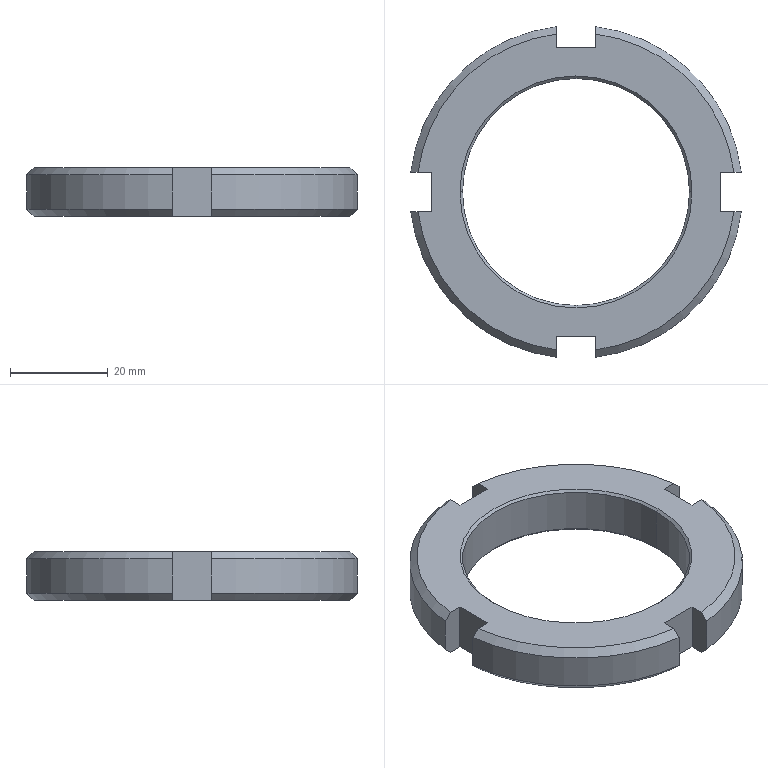Part | SolidWorks | features BaseBody 1 | 1 solid | 32 faces | box 67.528 x 67.528 x 10 mm | volume 17576 mm3 | plane 14 | cone 12 | cylinder 6 | commonest cylinder face diameters 68 x4 46.376 x2
STEP:
#1=CARTESIAN_POINT('',(-23.188,0.,9.5));
#2=VERTEX_POINT('',#1);
#3=CARTESIAN_POINT('',(23.188,0.,9.5));
#4=VERTEX_POINT('',#3);
#5=CARTESIAN_POINT('',(0.,0.,9.5));
#6=DIRECTION('',(0.,0.,1.));
#7=DIRECTION('',(1.,0.,0.));
#8=AXIS2_PLACEMENT_3D('',#5,#6,#7);
#9=CIRCLE('',#8,23.188);
#10=EDGE_CURVE('',#2,#4,#9,.T.);
#11=ORIENTED_EDGE('',*,*,#10,.F.);
#12=CARTESIAN_POINT('',(-23.688,0.,10.));
#13=VERTEX_POINT('',#12);
#14=CARTESIAN_POINT('',(-23.188,0.,9.5));
#15=DIRECTION('',(-0.7071,0.,0.7071));
#16=VECTOR('',#15,1000.);
#17=LINE('',#14,#16);
#18=EDGE_CURVE('',#2,#13,#17,.T.);
#19=ORIENTED_EDGE('',*,*,#18,.T.);
#20=CARTESIAN_POINT('',(23.688,0.,10.));
#21=VERTEX_POINT('',#20);
#22=CARTESIAN_POINT('',(0.,0.,10.));
#23=DIRECTION('',(0.,0.,-1.));
#24=DIRECTION('',(1.,0.,0.));
#25=AXIS2_PLACEMENT_3D('',#22,#23,#24);
#26=CIRCLE('',#25,23.688);
#27=EDGE_CURVE('',#21,#13,#26,.T.);
#28=ORIENTED_EDGE('',*,*,#27,.F.);
#29=CARTESIAN_POINT('',(23.188,0.,9.5));
#30=DIRECTION('',(0.7071,0.,0.7071));
#31=VECTOR('',#30,1000.);
#32=LINE('',#29,#31);
#33=EDGE_CURVE('',#4,#21,#32,.T.);
#34=ORIENTED_EDGE('',*,*,#33,.F.);
#35=EDGE_LOOP('',(#11,#19,#28,#34));
#36=FACE_OUTER_BOUND('',#35,.T.);
#37=CARTESIAN_POINT('',(0.,0.,9.5));
#38=DIRECTION('',(0.,0.,1.));
#39=DIRECTION('',(1.,0.,0.));
#40=AXIS2_PLACEMENT_3D('',#37,#38,#39);
#41=CONICAL_SURFACE('',#40,23.188,0.7854);
#42=ADVANCED_FACE('',(#36),#41,.F.);
#43=CARTESIAN_POINT('',(23.188,0.,0.5));
#44=VERTEX_POINT('',#43);
#45=CARTESIAN_POINT('',(-23.188,0.,0.5));
#46=VERTEX_POINT('',#45);
#47=CARTESIAN_POINT('',(0.,0.,0.5));
#48=DIRECTION('',(0.,0.,-1.));
#49=DIRECTION('',(1.,0.,0.));
#50=AXIS2_PLACEMENT_3D('',#47,#48,#49);
#51=CIRCLE('',#50,23.188);
#52=EDGE_CURVE('',#44,#46,#51,.T.);
#53=ORIENTED_EDGE('',*,*,#52,.F.);
#54=CARTESIAN_POINT('',(23.688,0.,0.));
#55=VERTEX_POINT('',#54);
#56=CARTESIAN_POINT('',(23.688,0.,0.));
#57=DIRECTION('',(0.7071,0.,-0.7071));
#58=VECTOR('',#57,1000.);
#59=LINE('',#56,#58);
#60=EDGE_CURVE('',#44,#55,#59,.T.);
#61=ORIENTED_EDGE('',*,*,#60,.T.);
#62=CARTESIAN_POINT('',(-23.688,0.,0.));
#63=VERTEX_POINT('',#62);
#64=CARTESIAN_POINT('',(0.,0.,0.));
#65=DIRECTION('',(0.,0.,1.));
#66=DIRECTION('',(1.,0.,0.));
#67=AXIS2_PLACEMENT_3D('',#64,#65,#66);
#68=CIRCLE('',#67,23.688);
#69=EDGE_CURVE('',#63,#55,#68,.T.);
#70=ORIENTED_EDGE('',*,*,#69,.F.);
#71=CARTESIAN_POINT('',(-23.688,0.,0.));
#72=DIRECTION('',(-0.7071,0.,-0.7071));
#73=VECTOR('',#72,1000.);
#74=LINE('',#71,#73);
#75=EDGE_CURVE('',#46,#63,#74,.T.);
#76=ORIENTED_EDGE('',*,*,#75,.F.);
#77=EDGE_LOOP('',(#53,#61,#70,#76));
#78=FACE_OUTER_BOUND('',#77,.T.);
#79=CARTESIAN_POINT('',(0.,0.,0.));
#80=DIRECTION('',(0.,0.,-1.));
#81=DIRECTION('',(-1.,0.,0.));
#82=AXIS2_PLACEMENT_3D('',#79,#80,#81);
#83=CONICAL_SURFACE('',#82,23.688,0.7854);
#84=ADVANCED_FACE('',(#78),#83,.F.);
#85=ORIENTED_EDGE('',*,*,#10,.T.);
#86=CARTESIAN_POINT('',(23.188,0.,10.));
#87=DIRECTION('',(0.,0.,-1.));
#88=VECTOR('',#87,1000.);
#89=LINE('',#86,#88);
#90=EDGE_CURVE('',#4,#44,#89,.T.);
#91=ORIENTED_EDGE('',*,*,#90,.T.);
#92=ORIENTED_EDGE('',*,*,#52,.T.);
#93=CARTESIAN_POINT('',(-23.188,0.,10.));
#94=DIRECTION('',(0.,0.,-1.));
#95=VECTOR('',#94,1000.);
#96=LINE('',#93,#95);
#97=EDGE_CURVE('',#2,#46,#96,.T.);
#98=ORIENTED_EDGE('',*,*,#97,.F.);
#99=EDGE_LOOP('',(#85,#91,#92,#98));
#100=FACE_OUTER_BOUND('',#99,.T.);
#101=CARTESIAN_POINT('',(0.,0.,10.));
#102=DIRECTION('',(0.,0.,-1.));
#103=DIRECTION('',(-1.,0.,0.));
#104=AXIS2_PLACEMENT_3D('',#101,#102,#103);
#105=CYLINDRICAL_SURFACE('',#104,23.188);
#106=ADVANCED_FACE('',(#100),#105,.F.);
#107=CARTESIAN_POINT('',(4.,33.764,8.5));
#108=VERTEX_POINT('',#107);
#109=CARTESIAN_POINT('',(33.764,4.,8.5));
#110=VERTEX_POINT('',#109);
#111=CARTESIAN_POINT('',(0.,0.,8.5));
#112=DIRECTION('',(0.,0.,-1.));
#113=DIRECTION('',(1.,0.,0.));
#114=AXIS2_PLACEMENT_3D('',#111,#112,#113);
#115=CIRCLE('',#114,34.);
#116=EDGE_CURVE('',#108,#110,#115,.T.);
#117=ORIENTED_EDGE('',*,*,#116,.T.);
#118=CARTESIAN_POINT('',(33.764,4.,1.5));
#119=VERTEX_POINT('',#118);
#120=CARTESIAN_POINT('',(33.764,4.,0.));
#121=DIRECTION('',(0.,0.,1.));
#122=VECTOR('',#121,1000.);
#123=LINE('',#120,#122);
#124=EDGE_CURVE('',#119,#110,#123,.T.);
#125=ORIENTED_EDGE('',*,*,#124,.F.);
#126=CARTESIAN_POINT('',(4.,33.764,1.5));
#127=VERTEX_POINT('',#126);
#128=CARTESIAN_POINT('',(0.,0.,1.5));
#129=DIRECTION('',(0.,0.,1.));
#130=DIRECTION('',(1.,0.,0.));
#131=AXIS2_PLACEMENT_3D('',#128,#129,#130);
#132=CIRCLE('',#131,34.);
#133=EDGE_CURVE('',#119,#127,#132,.T.);
#134=ORIENTED_EDGE('',*,*,#133,.T.);
#135=CARTESIAN_POINT('',(4.,33.764,0.));
#136=DIRECTION('',(0.,0.,1.));
#137=VECTOR('',#136,1000.);
#138=LINE('',#135,#137);
#139=EDGE_CURVE('',#127,#108,#138,.T.);
#140=ORIENTED_EDGE('',*,*,#139,.T.);
#141=EDGE_LOOP('',(#117,#125,#134,#140));
#142=FACE_OUTER_BOUND('',#141,.T.);
#143=CARTESIAN_POINT('',(0.,0.,10.));
#144=DIRECTION('',(0.,0.,-1.));
#145=DIRECTION('',(-1.,0.,0.));
#146=AXIS2_PLACEMENT_3D('',#143,#144,#145);
#147=CYLINDRICAL_SURFACE('',#146,34.);
#148=ADVANCED_FACE('',(#142),#147,.T.);
#149=CARTESIAN_POINT('',(32.253,4.,10.));
#150=VERTEX_POINT('',#149);
#151=CARTESIAN_POINT('',(33.764,4.,8.5));
#152=CARTESIAN_POINT('',(33.371,4.,8.89));
#153=CARTESIAN_POINT('',(32.979,4.,9.28));
#154=CARTESIAN_POINT('',(32.586,4.,9.669));
#155=CARTESIAN_POINT('',(32.475,4.,9.779));
#156=CARTESIAN_POINT('',(32.364,4.,9.89));
#157=CARTESIAN_POINT('',(32.253,4.,10.));
#158=B_SPLINE_CURVE_WITH_KNOTS('',3,(#151,#152,#153,#154,#155,#156,#157),.UNSPECIFIED.,.F.,.F.,(4,3,4),(0.007216,0.008875,0.009345),.UNSPECIFIED.);
#159=EDGE_CURVE('',#110,#150,#158,.T.);
#160=ORIENTED_EDGE('',*,*,#159,.F.);
#161=ORIENTED_EDGE('',*,*,#116,.F.);
#162=CARTESIAN_POINT('',(4.,32.253,10.));
#163=VERTEX_POINT('',#162);
#164=CARTESIAN_POINT('',(4.,32.253,10.));
#165=CARTESIAN_POINT('',(4.,32.364,9.89));
#166=CARTESIAN_POINT('',(4.,32.475,9.779));
#167=CARTESIAN_POINT('',(4.,32.586,9.669));
#168=CARTESIAN_POINT('',(4.,32.979,9.28));
#169=CARTESIAN_POINT('',(4.,33.371,8.89));
#170=CARTESIAN_POINT('',(4.,33.764,8.5));
#171=B_SPLINE_CURVE_WITH_KNOTS('',3,(#164,#165,#166,#167,#168,#169,#170),.UNSPECIFIED.,.F.,.F.,(4,3,4),(0.008406,0.008875,0.01053),.UNSPECIFIED.);
#172=EDGE_CURVE('',#163,#108,#171,.T.);
#173=ORIENTED_EDGE('',*,*,#172,.F.);
#174=CARTESIAN_POINT('',(0.,0.,10.));
#175=DIRECTION('',(0.,0.,1.));
#176=DIRECTION('',(1.,0.,0.));
#177=AXIS2_PLACEMENT_3D('',#174,#175,#176);
#178=CIRCLE('',#177,32.5);
#179=EDGE_CURVE('',#150,#163,#178,.T.);
#180=ORIENTED_EDGE('',*,*,#179,.F.);
#181=EDGE_LOOP('',(#160,#161,#173,#180));
#182=FACE_OUTER_BOUND('',#181,.T.);
#183=CARTESIAN_POINT('',(0.,0.,10.));
#184=DIRECTION('',(0.,0.,-1.));
#185=DIRECTION('',(-1.,0.,0.));
#186=AXIS2_PLACEMENT_3D('',#183,#184,#185);
#187=CONICAL_SURFACE('',#186,32.5,0.7854);
#188=ADVANCED_FACE('',(#182),#187,.T.);
#189=CARTESIAN_POINT('',(32.253,4.,0.));
#190=VERTEX_POINT('',#189);
#191=CARTESIAN_POINT('',(32.253,4.,0.));
#192=CARTESIAN_POINT('',(32.364,4.,0.1102));
#193=CARTESIAN_POINT('',(32.475,4.,0.2205));
#194=CARTESIAN_POINT('',(32.586,4.,0.3308));
#195=CARTESIAN_POINT('',(32.979,4.,0.7205));
#196=CARTESIAN_POINT('',(33.371,4.,1.11));
#197=CARTESIAN_POINT('',(33.764,4.,1.5));
#198=B_SPLINE_CURVE_WITH_KNOTS('',3,(#191,#192,#193,#194,#195,#196,#197),.UNSPECIFIED.,.F.,.F.,(4,3,4),(0.008406,0.008875,0.01053),.UNSPECIFIED.);
#199=EDGE_CURVE('',#190,#119,#198,.T.);
#200=ORIENTED_EDGE('',*,*,#199,.F.);
#201=CARTESIAN_POINT('',(4.,32.253,0.));
#202=VERTEX_POINT('',#201);
#203=CARTESIAN_POINT('',(0.,0.,0.));
#204=DIRECTION('',(0.,0.,-1.));
#205=DIRECTION('',(1.,0.,0.));
#206=AXIS2_PLACEMENT_3D('',#203,#204,#205);
#207=CIRCLE('',#206,32.5);
#208=EDGE_CURVE('',#202,#190,#207,.T.);
#209=ORIENTED_EDGE('',*,*,#208,.F.);
#210=CARTESIAN_POINT('',(4.,33.764,1.5));
#211=CARTESIAN_POINT('',(4.,33.371,1.11));
#212=CARTESIAN_POINT('',(4.,32.979,0.7205));
#213=CARTESIAN_POINT('',(4.,32.586,0.3308));
#214=CARTESIAN_POINT('',(4.,32.475,0.2205));
#215=CARTESIAN_POINT('',(4.,32.364,0.1102));
#216=CARTESIAN_POINT('',(4.,32.253,0.));
#217=B_SPLINE_CURVE_WITH_KNOTS('',3,(#210,#211,#212,#213,#214,#215,#216),.UNSPECIFIED.,.F.,.F.,(4,3,4),(0.007216,0.008875,0.009345),.UNSPECIFIED.);
#218=EDGE_CURVE('',#127,#202,#217,.T.);
#219=ORIENTED_EDGE('',*,*,#218,.F.);
#220=ORIENTED_EDGE('',*,*,#133,.F.);
#221=EDGE_LOOP('',(#200,#209,#219,#220));
#222=FACE_OUTER_BOUND('',#221,.T.);
#223=CARTESIAN_POINT('',(0.,0.,1.5));
#224=DIRECTION('',(0.,0.,1.));
#225=DIRECTION('',(1.,0.,0.));
#226=AXIS2_PLACEMENT_3D('',#223,#224,#225);
#227=CONICAL_SURFACE('',#226,34.,0.7854);
#228=ADVANCED_FACE('',(#222),#227,.T.);
#229=CARTESIAN_POINT('',(-33.764,4.,8.5));
#230=VERTEX_POINT('',#229);
#231=CARTESIAN_POINT('',(-4.,33.764,8.5));
#232=VERTEX_POINT('',#231);
#233=CARTESIAN_POINT('',(0.,0.,8.5));
#234=DIRECTION('',(0.,0.,-1.));
#235=DIRECTION('',(1.,0.,0.));
#236=AXIS2_PLACEMENT_3D('',#233,#234,#235);
#237=CIRCLE('',#236,34.);
#238=EDGE_CURVE('',#230,#232,#237,.T.);
#239=ORIENTED_EDGE('',*,*,#238,.T.);
#240=CARTESIAN_POINT('',(-4.,33.764,1.5));
#241=VERTEX_POINT('',#240);
#242=CARTESIAN_POINT('',(-4.,33.764,0.));
#243=DIRECTION('',(0.,0.,1.));
#244=VECTOR('',#243,1000.);
#245=LINE('',#242,#244);
#246=EDGE_CURVE('',#241,#232,#245,.T.);
#247=ORIENTED_EDGE('',*,*,#246,.F.);
#248=CARTESIAN_POINT('',(-33.764,4.,1.5));
#249=VERTEX_POINT('',#248);
#250=CARTESIAN_POINT('',(0.,0.,1.5));
#251=DIRECTION('',(0.,0.,1.));
#252=DIRECTION('',(1.,0.,0.));
#253=AXIS2_PLACEMENT_3D('',#250,#251,#252);
#254=CIRCLE('',#253,34.);
#255=EDGE_CURVE('',#241,#249,#254,.T.);
#256=ORIENTED_EDGE('',*,*,#255,.T.);
#257=CARTESIAN_POINT('',(-33.764,4.,0.));
#258=DIRECTION('',(0.,0.,1.));
#259=VECTOR('',#258,1000.);
#260=LINE('',#257,#259);
#261=EDGE_CURVE('',#249,#230,#260,.T.);
#262=ORIENTED_EDGE('',*,*,#261,.T.);
#263=EDGE_LOOP('',(#239,#247,#256,#262));
#264=FACE_OUTER_BOUND('',#263,.T.);
#265=CARTESIAN_POINT('',(0.,0.,10.));
#266=DIRECTION('',(0.,0.,-1.));
#267=DIRECTION('',(-1.,0.,0.));
#268=AXIS2_PLACEMENT_3D('',#265,#266,#267);
#269=CYLINDRICAL_SURFACE('',#268,34.);
#270=ADVANCED_FACE('',(#264),#269,.T.);
#271=CARTESIAN_POINT('',(-4.,32.253,10.));
#272=VERTEX_POINT('',#271);
#273=CARTESIAN_POINT('',(-4.,33.764,8.5));
#274=CARTESIAN_POINT('',(-4.,33.371,8.89));
#275=CARTESIAN_POINT('',(-4.,32.979,9.28));
#276=CARTESIAN_POINT('',(-4.,32.586,9.669));
#277=CARTESIAN_POINT('',(-4.,32.475,9.779));
#278=CARTESIAN_POINT('',(-4.,32.364,9.89));
#279=CARTESIAN_POINT('',(-4.,32.253,10.));
#280=B_SPLINE_CURVE_WITH_KNOTS('',3,(#273,#274,#275,#276,#277,#278,#279),.UNSPECIFIED.,.F.,.F.,(4,3,4),(0.007216,0.008875,0.009345),.UNSPECIFIED.);
#281=EDGE_CURVE('',#232,#272,#280,.T.);
#282=ORIENTED_EDGE('',*,*,#281,.F.);
#283=ORIENTED_EDGE('',*,*,#238,.F.);
#284=CARTESIAN_POINT('',(-32.253,4.,10.));
#285=VERTEX_POINT('',#284);
#286=CARTESIAN_POINT('',(-32.253,4.,10.));
#287=CARTESIAN_POINT('',(-32.542,4.,9.713));
#288=CARTESIAN_POINT('',(-32.832,4.,9.425));
#289=CARTESIAN_POINT('',(-33.121,4.,9.138));
#290=CARTESIAN_POINT('',(-33.336,4.,8.925));
#291=CARTESIAN_POINT('',(-33.55,4.,8.713));
#292=CARTESIAN_POINT('',(-33.764,4.,8.5));
#293=B_SPLINE_CURVE_WITH_KNOTS('',3,(#286,#287,#288,#289,#290,#291,#292),.UNSPECIFIED.,.F.,.F.,(4,3,4),(0.007652,0.008875,0.009781),.UNSPECIFIED.);
#294=EDGE_CURVE('',#285,#230,#293,.T.);
#295=ORIENTED_EDGE('',*,*,#294,.F.);
#296=CARTESIAN_POINT('',(0.,0.,10.));
#297=DIRECTION('',(0.,0.,1.));
#298=DIRECTION('',(1.,0.,0.));
#299=AXIS2_PLACEMENT_3D('',#296,#297,#298);
#300=CIRCLE('',#299,32.5);
#301=EDGE_CURVE('',#272,#285,#300,.T.);
#302=ORIENTED_EDGE('',*,*,#301,.F.);
#303=EDGE_LOOP('',(#282,#283,#295,#302));
#304=FACE_OUTER_BOUND('',#303,.T.);
#305=CARTESIAN_POINT('',(0.,0.,10.));
#306=DIRECTION('',(0.,0.,-1.));
#307=DIRECTION('',(-1.,0.,0.));
#308=AXIS2_PLACEMENT_3D('',#305,#306,#307);
#309=CONICAL_SURFACE('',#308,32.5,0.7854);
#310=ADVANCED_FACE('',(#304),#309,.T.);
#311=CARTESIAN_POINT('',(-4.,32.253,0.));
#312=VERTEX_POINT('',#311);
#313=CARTESIAN_POINT('',(-4.,32.253,0.));
#314=CARTESIAN_POINT('',(-4.,32.364,0.1102));
#315=CARTESIAN_POINT('',(-4.,32.475,0.2205));
#316=CARTESIAN_POINT('',(-4.,32.586,0.3308));
#317=CARTESIAN_POINT('',(-4.,32.979,0.7205));
#318=CARTESIAN_POINT('',(-4.,33.371,1.11));
#319=CARTESIAN_POINT('',(-4.,33.764,1.5));
#320=B_SPLINE_CURVE_WITH_KNOTS('',3,(#313,#314,#315,#316,#317,#318,#319),.UNSPECIFIED.,.F.,.F.,(4,3,4),(0.008406,0.008875,0.01053),.UNSPECIFIED.);
#321=EDGE_CURVE('',#312,#241,#320,.T.);
#322=ORIENTED_EDGE('',*,*,#321,.F.);
#323=CARTESIAN_POINT('',(-32.253,4.,0.));
#324=VERTEX_POINT('',#323);
#325=CARTESIAN_POINT('',(0.,0.,0.));
#326=DIRECTION('',(0.,0.,-1.));
#327=DIRECTION('',(1.,0.,0.));
#328=AXIS2_PLACEMENT_3D('',#325,#326,#327);
#329=CIRCLE('',#328,32.5);
#330=EDGE_CURVE('',#324,#312,#329,.T.);
#331=ORIENTED_EDGE('',*,*,#330,.F.);
#332=CARTESIAN_POINT('',(-33.764,4.,1.5));
#333=CARTESIAN_POINT('',(-33.55,4.,1.287));
#334=CARTESIAN_POINT('',(-33.336,4.,1.075));
#335=CARTESIAN_POINT('',(-33.121,4.,0.8621));
#336=CARTESIAN_POINT('',(-32.832,4.,0.5747));
#337=CARTESIAN_POINT('',(-32.542,4.,0.2873));
#338=CARTESIAN_POINT('',(-32.253,4.,0.));
#339=B_SPLINE_CURVE_WITH_KNOTS('',3,(#332,#333,#334,#335,#336,#337,#338),.UNSPECIFIED.,.F.,.F.,(4,3,4),(0.00797,0.008875,0.0101),.UNSPECIFIED.);
#340=EDGE_CURVE('',#249,#324,#339,.T.);
#341=ORIENTED_EDGE('',*,*,#340,.F.);
#342=ORIENTED_EDGE('',*,*,#255,.F.);
#343=EDGE_LOOP('',(#322,#331,#341,#342));
#344=FACE_OUTER_BOUND('',#343,.T.);
#345=CARTESIAN_POINT('',(0.,0.,1.5));
#346=DIRECTION('',(0.,0.,1.));
#347=DIRECTION('',(1.,0.,0.));
#348=AXIS2_PLACEMENT_3D('',#345,#346,#347);
#349=CONICAL_SURFACE('',#348,34.,0.7854);
#350=ADVANCED_FACE('',(#344),#349,.T.);
#351=CARTESIAN_POINT('',(-4.,-33.764,8.5));
#352=VERTEX_POINT('',#351);
#353=CARTESIAN_POINT('',(-33.764,-4.,8.5));
#354=VERTEX_POINT('',#353);
#355=CARTESIAN_POINT('',(0.,0.,8.5));
#356=DIRECTION('',(0.,0.,-1.));
#357=DIRECTION('',(1.,0.,0.));
#358=AXIS2_PLACEMENT_3D('',#355,#356,#357);
#359=CIRCLE('',#358,34.);
#360=EDGE_CURVE('',#352,#354,#359,.T.);
#361=ORIENTED_EDGE('',*,*,#360,.T.);
#362=CARTESIAN_POINT('',(-33.764,-4.,1.5));
#363=VERTEX_POINT('',#362);
#364=CARTESIAN_POINT('',(-33.764,-4.,0.));
#365=DIRECTION('',(0.,0.,1.));
#366=VECTOR('',#365,1000.);
#367=LINE('',#364,#366);
#368=EDGE_CURVE('',#363,#354,#367,.T.);
#369=ORIENTED_EDGE('',*,*,#368,.F.);
#370=CARTESIAN_POINT('',(-4.,-33.764,1.5));
#371=VERTEX_POINT('',#370);
#372=CARTESIAN_POINT('',(0.,0.,1.5));
#373=DIRECTION('',(0.,0.,1.));
#374=DIRECTION('',(1.,0.,0.));
#375=AXIS2_PLACEMENT_3D('',#372,#373,#374);
#376=CIRCLE('',#375,34.);
#377=EDGE_CURVE('',#363,#371,#376,.T.);
#378=ORIENTED_EDGE('',*,*,#377,.T.);
#379=CARTESIAN_POINT('',(-4.,-33.764,0.));
#380=DIRECTION('',(0.,0.,1.));
#381=VECTOR('',#380,1000.);
#382=LINE('',#379,#381);
#383=EDGE_CURVE('',#371,#352,#382,.T.);
#384=ORIENTED_EDGE('',*,*,#383,.T.);
#385=EDGE_LOOP('',(#361,#369,#378,#384));
#386=FACE_OUTER_BOUND('',#385,.T.);
#387=CARTESIAN_POINT('',(0.,0.,10.));
#388=DIRECTION('',(0.,0.,-1.));
#389=DIRECTION('',(-1.,0.,0.));
#390=AXIS2_PLACEMENT_3D('',#387,#388,#389);
#391=CYLINDRICAL_SURFACE('',#390,34.);
#392=ADVANCED_FACE('',(#386),#391,.T.);
#393=CARTESIAN_POINT('',(-32.253,-4.,10.));
#394=VERTEX_POINT('',#393);
#395=CARTESIAN_POINT('',(-33.764,-4.,8.5));
#396=CARTESIAN_POINT('',(-33.55,-4.,8.713));
#397=CARTESIAN_POINT('',(-33.336,-4.,8.925));
#398=CARTESIAN_POINT('',(-33.121,-4.,9.138));
#399=CARTESIAN_POINT('',(-32.832,-4.,9.425));
#400=CARTESIAN_POINT('',(-32.542,-4.,9.713));
#401=CARTESIAN_POINT('',(-32.253,-4.,10.));
#402=B_SPLINE_CURVE_WITH_KNOTS('',3,(#395,#396,#397,#398,#399,#400,#401),.UNSPECIFIED.,.F.,.F.,(4,3,4),(0.00797,0.008875,0.0101),.UNSPECIFIED.);
#403=EDGE_CURVE('',#354,#394,#402,.T.);
#404=ORIENTED_EDGE('',*,*,#403,.F.);
#405=ORIENTED_EDGE('',*,*,#360,.F.);
#406=CARTESIAN_POINT('',(-4.,-32.253,10.));
#407=VERTEX_POINT('',#406);
#408=CARTESIAN_POINT('',(-4.,-32.253,10.));
#409=CARTESIAN_POINT('',(-4.,-32.757,9.5));
#410=CARTESIAN_POINT('',(-4.,-33.26,9.));
#411=CARTESIAN_POINT('',(-4.,-33.764,8.5));
#412=B_SPLINE_CURVE_WITH_KNOTS('',3,(#408,#409,#410,#411),.UNSPECIFIED.,.F.,.F.,(4,4),(0.,0.002129),.UNSPECIFIED.);
#413=EDGE_CURVE('',#407,#352,#412,.T.);
#414=ORIENTED_EDGE('',*,*,#413,.F.);
#415=CARTESIAN_POINT('',(0.,0.,10.));
#416=DIRECTION('',(0.,0.,1.));
#417=DIRECTION('',(1.,0.,0.));
#418=AXIS2_PLACEMENT_3D('',#415,#416,#417);
#419=CIRCLE('',#418,32.5);
#420=EDGE_CURVE('',#394,#407,#419,.T.);
#421=ORIENTED_EDGE('',*,*,#420,.F.);
#422=EDGE_LOOP('',(#404,#405,#414,#421));
#423=FACE_OUTER_BOUND('',#422,.T.);
#424=CARTESIAN_POINT('',(0.,0.,10.));
#425=DIRECTION('',(0.,0.,-1.));
#426=DIRECTION('',(-1.,0.,0.));
#427=AXIS2_PLACEMENT_3D('',#424,#425,#426);
#428=CONICAL_SURFACE('',#427,32.5,0.7854);
#429=ADVANCED_FACE('',(#423),#428,.T.);
#430=CARTESIAN_POINT('',(-32.253,-4.,0.));
#431=VERTEX_POINT('',#430);
#432=CARTESIAN_POINT('',(-32.253,-4.,0.));
#433=CARTESIAN_POINT('',(-32.542,-4.,0.2873));
#434=CARTESIAN_POINT('',(-32.832,-4.,0.5747));
#435=CARTESIAN_POINT('',(-33.121,-4.,0.8621));
#436=CARTESIAN_POINT('',(-33.336,-4.,1.075));
#437=CARTESIAN_POINT('',(-33.55,-4.,1.287));
#438=CARTESIAN_POINT('',(-33.764,-4.,1.5));
#439=B_SPLINE_CURVE_WITH_KNOTS('',3,(#432,#433,#434,#435,#436,#437,#438),.UNSPECIFIED.,.F.,.F.,(4,3,4),(0.007652,0.008875,0.009781),.UNSPECIFIED.);
#440=EDGE_CURVE('',#431,#363,#439,.T.);
#441=ORIENTED_EDGE('',*,*,#440,.F.);
#442=CARTESIAN_POINT('',(-4.,-32.253,0.));
#443=VERTEX_POINT('',#442);
#444=CARTESIAN_POINT('',(0.,0.,0.));
#445=DIRECTION('',(0.,0.,-1.));
#446=DIRECTION('',(1.,0.,0.));
#447=AXIS2_PLACEMENT_3D('',#444,#445,#446);
#448=CIRCLE('',#447,32.5);
#449=EDGE_CURVE('',#443,#431,#448,.T.);
#450=ORIENTED_EDGE('',*,*,#449,.F.);
#451=CARTESIAN_POINT('',(-4.,-33.764,1.5));
#452=CARTESIAN_POINT('',(-4.,-33.26,0.9999));
#453=CARTESIAN_POINT('',(-4.,-32.757,0.4999));
#454=CARTESIAN_POINT('',(-4.,-32.253,0.));
#455=B_SPLINE_CURVE_WITH_KNOTS('',3,(#451,#452,#453,#454),.UNSPECIFIED.,.F.,.F.,(4,4),(0.,0.002129),.UNSPECIFIED.);
#456=EDGE_CURVE('',#371,#443,#455,.T.);
#457=ORIENTED_EDGE('',*,*,#456,.F.);
#458=ORIENTED_EDGE('',*,*,#377,.F.);
#459=EDGE_LOOP('',(#441,#450,#457,#458));
#460=FACE_OUTER_BOUND('',#459,.T.);
#461=CARTESIAN_POINT('',(0.,0.,1.5));
#462=DIRECTION('',(0.,0.,1.));
#463=DIRECTION('',(1.,0.,0.));
#464=AXIS2_PLACEMENT_3D('',#461,#462,#463);
#465=CONICAL_SURFACE('',#464,34.,0.7854);
#466=ADVANCED_FACE('',(#460),#465,.T.);
#467=ORIENTED_EDGE('',*,*,#27,.T.);
#468=CARTESIAN_POINT('',(0.,0.,10.));
#469=DIRECTION('',(0.,0.,-1.));
#470=DIRECTION('',(1.,0.,0.));
#471=AXIS2_PLACEMENT_3D('',#468,#469,#470);
#472=CIRCLE('',#471,23.688);
#473=EDGE_CURVE('',#13,#21,#472,.T.);
#474=ORIENTED_EDGE('',*,*,#473,.T.);
#475=EDGE_LOOP('',(#467,#474));
#476=FACE_BOUND('',#475,.T.);
#477=CARTESIAN_POINT('',(29.514,4.,10.));
#478=VERTEX_POINT('',#477);
#479=CARTESIAN_POINT('',(29.514,4.,10.));
#480=DIRECTION('',(-1.,0.,0.));
#481=VECTOR('',#480,1000.);
#482=LINE('',#479,#481);
#483=EDGE_CURVE('',#150,#478,#482,.T.);
#484=ORIENTED_EDGE('',*,*,#483,.F.);
#485=ORIENTED_EDGE('',*,*,#179,.T.);
#486=CARTESIAN_POINT('',(4.,29.514,10.));
#487=VERTEX_POINT('',#486);
#488=CARTESIAN_POINT('',(4.,29.514,10.));
#489=DIRECTION('',(0.,1.,0.));
#490=VECTOR('',#489,1000.);
#491=LINE('',#488,#490);
#492=EDGE_CURVE('',#487,#163,#491,.T.);
#493=ORIENTED_EDGE('',*,*,#492,.F.);
#494=CARTESIAN_POINT('',(-4.,29.514,10.));
#495=VERTEX_POINT('',#494);
#496=CARTESIAN_POINT('',(4.,29.514,10.));
#497=DIRECTION('',(1.,0.,0.));
#498=VECTOR('',#497,1000.);
#499=LINE('',#496,#498);
#500=EDGE_CURVE('',#495,#487,#499,.T.);
#501=ORIENTED_EDGE('',*,*,#500,.F.);
#502=CARTESIAN_POINT('',(-4.,29.514,10.));
#503=DIRECTION('',(0.,-1.,0.));
#504=VECTOR('',#503,1000.);
#505=LINE('',#502,#504);
#506=EDGE_CURVE('',#272,#495,#505,.T.);
#507=ORIENTED_EDGE('',*,*,#506,.F.);
#508=ORIENTED_EDGE('',*,*,#301,.T.);
#509=CARTESIAN_POINT('',(-29.514,4.,10.));
#510=VERTEX_POINT('',#509);
#511=CARTESIAN_POINT('',(-29.514,4.,10.));
#512=DIRECTION('',(-1.,0.,0.));
#513=VECTOR('',#512,1000.);
#514=LINE('',#511,#513);
#515=EDGE_CURVE('',#510,#285,#514,.T.);
#516=ORIENTED_EDGE('',*,*,#515,.F.);
#517=CARTESIAN_POINT('',(-29.514,-4.,10.));
#518=VERTEX_POINT('',#517);
#519=CARTESIAN_POINT('',(-29.514,4.,10.));
#520=DIRECTION('',(0.,1.,0.));
#521=VECTOR('',#520,1000.);
#522=LINE('',#519,#521);
#523=EDGE_CURVE('',#518,#510,#522,.T.);
#524=ORIENTED_EDGE('',*,*,#523,.F.);
#525=CARTESIAN_POINT('',(-29.514,-4.,10.));
#526=DIRECTION('',(1.,0.,0.));
#527=VECTOR('',#526,1000.);
#528=LINE('',#525,#527);
#529=EDGE_CURVE('',#394,#518,#528,.T.);
#530=ORIENTED_EDGE('',*,*,#529,.F.);
#531=ORIENTED_EDGE('',*,*,#420,.T.);
#532=CARTESIAN_POINT('',(-4.,-29.514,10.));
#533=VERTEX_POINT('',#532);
#534=CARTESIAN_POINT('',(-4.,-29.514,10.));
#535=DIRECTION('',(0.,-1.,0.));
#536=VECTOR('',#535,1000.);
#537=LINE('',#534,#536);
#538=EDGE_CURVE('',#533,#407,#537,.T.);
#539=ORIENTED_EDGE('',*,*,#538,.F.);
#540=CARTESIAN_POINT('',(4.,-29.514,10.));
#541=VERTEX_POINT('',#540);
#542=CARTESIAN_POINT('',(-4.,-29.514,10.));
#543=DIRECTION('',(-1.,0.,0.));
#544=VECTOR('',#543,1000.);
#545=LINE('',#542,#544);
#546=EDGE_CURVE('',#541,#533,#545,.T.);
#547=ORIENTED_EDGE('',*,*,#546,.F.);
#548=CARTESIAN_POINT('',(4.,-32.253,10.));
#549=VERTEX_POINT('',#548);
#550=CARTESIAN_POINT('',(4.,-29.514,10.));
#551=DIRECTION('',(0.,1.,0.));
#552=VECTOR('',#551,1000.);
#553=LINE('',#550,#552);
#554=EDGE_CURVE('',#549,#541,#553,.T.);
#555=ORIENTED_EDGE('',*,*,#554,.F.);
#556=CARTESIAN_POINT('',(32.253,-4.,10.));
#557=VERTEX_POINT('',#556);
#558=CARTESIAN_POINT('',(0.,0.,10.));
#559=DIRECTION('',(0.,0.,1.));
#560=DIRECTION('',(1.,0.,0.));
#561=AXIS2_PLACEMENT_3D('',#558,#559,#560);
#562=CIRCLE('',#561,32.5);
#563=EDGE_CURVE('',#549,#557,#562,.T.);
#564=ORIENTED_EDGE('',*,*,#563,.T.);
#565=CARTESIAN_POINT('',(29.514,-4.,10.));
#566=VERTEX_POINT('',#565);
#567=CARTESIAN_POINT('',(29.514,-4.,10.));
#568=DIRECTION('',(1.,0.,0.));
#569=VECTOR('',#568,1000.);
#570=LINE('',#567,#569);
#571=EDGE_CURVE('',#566,#557,#570,.T.);
#572=ORIENTED_EDGE('',*,*,#571,.F.);
#573=CARTESIAN_POINT('',(29.514,-4.,10.));
#574=DIRECTION('',(0.,-1.,0.));
#575=VECTOR('',#574,1000.);
#576=LINE('',#573,#575);
#577=EDGE_CURVE('',#478,#566,#576,.T.);
#578=ORIENTED_EDGE('',*,*,#577,.F.);
#579=EDGE_LOOP('',(#484,#485,#493,#501,#507,#508,#516,#524,#530,#531,#539,#547,#555,#564,#572,#578));
#580=FACE_OUTER_BOUND('',#579,.T.);
#581=CARTESIAN_POINT('',(0.,0.,10.));
#582=DIRECTION('',(0.,0.,1.));
#583=DIRECTION('',(1.,0.,0.));
#584=AXIS2_PLACEMENT_3D('',#581,#582,#583);
#585=PLANE('',#584);
#586=ADVANCED_FACE('',(#476,#580),#585,.T.);
#587=ORIENTED_EDGE('',*,*,#69,.T.);
#588=CARTESIAN_POINT('',(0.,0.,0.));
#589=DIRECTION('',(0.,0.,1.));
#590=DIRECTION('',(1.,0.,0.));
#591=AXIS2_PLACEMENT_3D('',#588,#589,#590);
#592=CIRCLE('',#591,23.688);
#593=EDGE_CURVE('',#55,#63,#592,.T.);
#594=ORIENTED_EDGE('',*,*,#593,.T.);
#595=EDGE_LOOP('',(#587,#594));
#596=FACE_BOUND('',#595,.T.);
#597=ORIENTED_EDGE('',*,*,#208,.T.);
#598=CARTESIAN_POINT('',(29.514,4.,0.));
#599=VERTEX_POINT('',#598);
#600=CARTESIAN_POINT('',(29.514,4.,0.));
#601=DIRECTION('',(-1.,0.,0.));
#602=VECTOR('',#601,1000.);
#603=LINE('',#600,#602);
#604=EDGE_CURVE('',#190,#599,#603,.T.);
#605=ORIENTED_EDGE('',*,*,#604,.T.);
#606=CARTESIAN_POINT('',(29.514,-4.,0.));
#607=VERTEX_POINT('',#606);
#608=CARTESIAN_POINT('',(29.514,-4.,0.));
#609=DIRECTION('',(0.,-1.,0.));
#610=VECTOR('',#609,1000.);
#611=LINE('',#608,#610);
#612=EDGE_CURVE('',#599,#607,#611,.T.);
#613=ORIENTED_EDGE('',*,*,#612,.T.);
#614=CARTESIAN_POINT('',(32.253,-4.,0.));
#615=VERTEX_POINT('',#614);
#616=CARTESIAN_POINT('',(29.514,-4.,0.));
#617=DIRECTION('',(1.,0.,0.));
#618=VECTOR('',#617,1000.);
#619=LINE('',#616,#618);
#620=EDGE_CURVE('',#607,#615,#619,.T.);
#621=ORIENTED_EDGE('',*,*,#620,.T.);
#622=CARTESIAN_POINT('',(4.,-32.253,0.));
#623=VERTEX_POINT('',#622);
#624=CARTESIAN_POINT('',(0.,0.,0.));
#625=DIRECTION('',(0.,0.,-1.));
#626=DIRECTION('',(1.,0.,0.));
#627=AXIS2_PLACEMENT_3D('',#624,#625,#626);
#628=CIRCLE('',#627,32.5);
#629=EDGE_CURVE('',#615,#623,#628,.T.);
#630=ORIENTED_EDGE('',*,*,#629,.T.);
#631=CARTESIAN_POINT('',(4.,-29.514,0.));
#632=VERTEX_POINT('',#631);
#633=CARTESIAN_POINT('',(4.,-29.514,0.));
#634=DIRECTION('',(0.,1.,0.));
#635=VECTOR('',#634,1000.);
#636=LINE('',#633,#635);
#637=EDGE_CURVE('',#623,#632,#636,.T.);
#638=ORIENTED_EDGE('',*,*,#637,.T.);
#639=CARTESIAN_POINT('',(-4.,-29.514,0.));
#640=VERTEX_POINT('',#639);
#641=CARTESIAN_POINT('',(-4.,-29.514,0.));
#642=DIRECTION('',(-1.,0.,0.));
#643=VECTOR('',#642,1000.);
#644=LINE('',#641,#643);
#645=EDGE_CURVE('',#632,#640,#644,.T.);
#646=ORIENTED_EDGE('',*,*,#645,.T.);
#647=CARTESIAN_POINT('',(-4.,-29.514,0.));
#648=DIRECTION('',(0.,-1.,0.));
#649=VECTOR('',#648,1000.);
#650=LINE('',#647,#649);
#651=EDGE_CURVE('',#640,#443,#650,.T.);
#652=ORIENTED_EDGE('',*,*,#651,.T.);
#653=ORIENTED_EDGE('',*,*,#449,.T.);
#654=CARTESIAN_POINT('',(-29.514,-4.,0.));
#655=VERTEX_POINT('',#654);
#656=CARTESIAN_POINT('',(-29.514,-4.,0.));
#657=DIRECTION('',(1.,0.,0.));
#658=VECTOR('',#657,1000.);
#659=LINE('',#656,#658);
#660=EDGE_CURVE('',#431,#655,#659,.T.);
#661=ORIENTED_EDGE('',*,*,#660,.T.);
#662=CARTESIAN_POINT('',(-29.514,4.,0.));
#663=VERTEX_POINT('',#662);
#664=CARTESIAN_POINT('',(-29.514,4.,0.));
#665=DIRECTION('',(0.,1.,0.));
#666=VECTOR('',#665,1000.);
#667=LINE('',#664,#666);
#668=EDGE_CURVE('',#655,#663,#667,.T.);
#669=ORIENTED_EDGE('',*,*,#668,.T.);
#670=CARTESIAN_POINT('',(-29.514,4.,0.));
#671=DIRECTION('',(-1.,0.,0.));
#672=VECTOR('',#671,1000.);
#673=LINE('',#670,#672);
#674=EDGE_CURVE('',#663,#324,#673,.T.);
#675=ORIENTED_EDGE('',*,*,#674,.T.);
#676=ORIENTED_EDGE('',*,*,#330,.T.);
#677=CARTESIAN_POINT('',(-4.,29.514,0.));
#678=VERTEX_POINT('',#677);
#679=CARTESIAN_POINT('',(-4.,29.514,0.));
#680=DIRECTION('',(0.,-1.,0.));
#681=VECTOR('',#680,1000.);
#682=LINE('',#679,#681);
#683=EDGE_CURVE('',#312,#678,#682,.T.);
#684=ORIENTED_EDGE('',*,*,#683,.T.);
#685=CARTESIAN_POINT('',(4.,29.514,0.));
#686=VERTEX_POINT('',#685);
#687=CARTESIAN_POINT('',(4.,29.514,0.));
#688=DIRECTION('',(1.,0.,0.));
#689=VECTOR('',#688,1000.);
#690=LINE('',#687,#689);
#691=EDGE_CURVE('',#678,#686,#690,.T.);
#692=ORIENTED_EDGE('',*,*,#691,.T.);
#693=CARTESIAN_POINT('',(4.,29.514,0.));
#694=DIRECTION('',(0.,1.,0.));
#695=VECTOR('',#694,1000.);
#696=LINE('',#693,#695);
#697=EDGE_CURVE('',#686,#202,#696,.T.);
#698=ORIENTED_EDGE('',*,*,#697,.T.);
#699=EDGE_LOOP('',(#597,#605,#613,#621,#630,#638,#646,#652,#653,#661,#669,#675,#676,#684,#692,#698));
#700=FACE_OUTER_BOUND('',#699,.T.);
#701=CARTESIAN_POINT('',(0.,0.,0.));
#702=DIRECTION('',(0.,0.,1.));
#703=DIRECTION('',(1.,0.,0.));
#704=AXIS2_PLACEMENT_3D('',#701,#702,#703);
#705=PLANE('',#704);
#706=ADVANCED_FACE('',(#596,#700),#705,.F.);
#707=CARTESIAN_POINT('',(4.,-33.764,1.5));
#708=VERTEX_POINT('',#707);
#709=CARTESIAN_POINT('',(33.764,-4.,1.5));
#710=VERTEX_POINT('',#709);
#711=CARTESIAN_POINT('',(0.,0.,1.5));
#712=DIRECTION('',(0.,0.,1.));
#713=DIRECTION('',(1.,0.,0.));
#714=AXIS2_PLACEMENT_3D('',#711,#712,#713);
#715=CIRCLE('',#714,34.);
#716=EDGE_CURVE('',#708,#710,#715,.T.);
#717=ORIENTED_EDGE('',*,*,#716,.T.);
#718=CARTESIAN_POINT('',(33.764,-4.,8.5));
#719=VERTEX_POINT('',#718);
#720=CARTESIAN_POINT('',(33.764,-4.,0.));
#721=DIRECTION('',(0.,0.,1.));
#722=VECTOR('',#721,1000.);
#723=LINE('',#720,#722);
#724=EDGE_CURVE('',#710,#719,#723,.T.);
#725=ORIENTED_EDGE('',*,*,#724,.T.);
#726=CARTESIAN_POINT('',(4.,-33.764,8.5));
#727=VERTEX_POINT('',#726);
#728=CARTESIAN_POINT('',(0.,0.,8.5));
#729=DIRECTION('',(0.,0.,-1.));
#730=DIRECTION('',(1.,0.,0.));
#731=AXIS2_PLACEMENT_3D('',#728,#729,#730);
#732=CIRCLE('',#731,34.);
#733=EDGE_CURVE('',#719,#727,#732,.T.);
#734=ORIENTED_EDGE('',*,*,#733,.T.);
#735=CARTESIAN_POINT('',(4.,-33.764,0.));
#736=DIRECTION('',(0.,0.,1.));
#737=VECTOR('',#736,1000.);
#738=LINE('',#735,#737);
#739=EDGE_CURVE('',#708,#727,#738,.T.);
#740=ORIENTED_EDGE('',*,*,#739,.F.);
#741=EDGE_LOOP('',(#717,#725,#734,#740));
#742=FACE_OUTER_BOUND('',#741,.T.);
#743=CARTESIAN_POINT('',(0.,0.,10.));
#744=DIRECTION('',(0.,0.,-1.));
#745=DIRECTION('',(-1.,0.,0.));
#746=AXIS2_PLACEMENT_3D('',#743,#744,#745);
#747=CYLINDRICAL_SURFACE('',#746,34.);
#748=ADVANCED_FACE('',(#742),#747,.T.);
#749=ORIENTED_EDGE('',*,*,#90,.F.);
#750=CARTESIAN_POINT('',(0.,0.,9.5));
#751=DIRECTION('',(0.,0.,1.));
#752=DIRECTION('',(1.,0.,0.));
#753=AXIS2_PLACEMENT_3D('',#750,#751,#752);
#754=CIRCLE('',#753,23.188);
#755=EDGE_CURVE('',#4,#2,#754,.T.);
#756=ORIENTED_EDGE('',*,*,#755,.T.);
#757=ORIENTED_EDGE('',*,*,#97,.T.);
#758=CARTESIAN_POINT('',(0.,0.,0.5));
#759=DIRECTION('',(0.,0.,-1.));
#760=DIRECTION('',(1.,0.,0.));
#761=AXIS2_PLACEMENT_3D('',#758,#759,#760);
#762=CIRCLE('',#761,23.188);
#763=EDGE_CURVE('',#46,#44,#762,.T.);
#764=ORIENTED_EDGE('',*,*,#763,.T.);
#765=EDGE_LOOP('',(#749,#756,#757,#764));
#766=FACE_OUTER_BOUND('',#765,.T.);
#767=CARTESIAN_POINT('',(0.,0.,10.));
#768=DIRECTION('',(0.,0.,-1.));
#769=DIRECTION('',(-1.,0.,0.));
#770=AXIS2_PLACEMENT_3D('',#767,#768,#769);
#771=CYLINDRICAL_SURFACE('',#770,23.188);
#772=ADVANCED_FACE('',(#766),#771,.F.);
#773=ORIENTED_EDGE('',*,*,#546,.T.);
#774=CARTESIAN_POINT('',(-4.,-29.514,0.));
#775=DIRECTION('',(0.,0.,1.));
#776=VECTOR('',#775,1000.);
#777=LINE('',#774,#776);
#778=EDGE_CURVE('',#640,#533,#777,.T.);
#779=ORIENTED_EDGE('',*,*,#778,.F.);
#780=ORIENTED_EDGE('',*,*,#645,.F.);
#781=CARTESIAN_POINT('',(4.,-29.514,0.));
#782=DIRECTION('',(0.,0.,1.));
#783=VECTOR('',#782,1000.);
#784=LINE('',#781,#783);
#785=EDGE_CURVE('',#632,#541,#784,.T.);
#786=ORIENTED_EDGE('',*,*,#785,.T.);
#787=EDGE_LOOP('',(#773,#779,#780,#786));
#788=FACE_OUTER_BOUND('',#787,.T.);
#789=CARTESIAN_POINT('',(-4.,-29.514,0.));
#790=DIRECTION('',(0.,1.,0.));
#791=DIRECTION('',(0.,0.,1.));
#792=AXIS2_PLACEMENT_3D('',#789,#790,#791);
#793=PLANE('',#792);
#794=ADVANCED_FACE('',(#788),#793,.F.);
#795=ORIENTED_EDGE('',*,*,#739,.T.);
#796=CARTESIAN_POINT('',(4.,-33.764,8.5));
#797=CARTESIAN_POINT('',(4.,-33.26,9.));
#798=CARTESIAN_POINT('',(4.,-32.757,9.5));
#799=CARTESIAN_POINT('',(4.,-32.253,10.));
#800=B_SPLINE_CURVE_WITH_KNOTS('',3,(#796,#797,#798,#799),.UNSPECIFIED.,.F.,.F.,(4,4),(0.,0.002129),.UNSPECIFIED.);
#801=EDGE_CURVE('',#727,#549,#800,.T.);
#802=ORIENTED_EDGE('',*,*,#801,.T.);
#803=ORIENTED_EDGE('',*,*,#554,.T.);
#804=ORIENTED_EDGE('',*,*,#785,.F.);
#805=ORIENTED_EDGE('',*,*,#637,.F.);
#806=CARTESIAN_POINT('',(4.,-32.253,0.));
#807=CARTESIAN_POINT('',(4.,-32.757,0.4999));
#808=CARTESIAN_POINT('',(4.,-33.26,0.9999));
#809=CARTESIAN_POINT('',(4.,-33.764,1.5));
#810=B_SPLINE_CURVE_WITH_KNOTS('',3,(#806,#807,#808,#809),.UNSPECIFIED.,.F.,.F.,(4,4),(0.,0.002129),.UNSPECIFIED.);
#811=EDGE_CURVE('',#623,#708,#810,.T.);
#812=ORIENTED_EDGE('',*,*,#811,.T.);
#813=EDGE_LOOP('',(#795,#802,#803,#804,#805,#812));
#814=FACE_OUTER_BOUND('',#813,.T.);
#815=CARTESIAN_POINT('',(4.,-29.514,0.));
#816=DIRECTION('',(1.,0.,0.));
#817=DIRECTION('',(0.,1.,0.));
#818=AXIS2_PLACEMENT_3D('',#815,#816,#817);
#819=PLANE('',#818);
#820=ADVANCED_FACE('',(#814),#819,.F.);
#821=ORIENTED_EDGE('',*,*,#538,.T.);
#822=ORIENTED_EDGE('',*,*,#413,.T.);
#823=ORIENTED_EDGE('',*,*,#383,.F.);
#824=ORIENTED_EDGE('',*,*,#456,.T.);
#825=ORIENTED_EDGE('',*,*,#651,.F.);
#826=ORIENTED_EDGE('',*,*,#778,.T.);
#827=EDGE_LOOP('',(#821,#822,#823,#824,#825,#826));
#828=FACE_OUTER_BOUND('',#827,.T.);
#829=CARTESIAN_POINT('',(-4.,-29.514,0.));
#830=DIRECTION('',(-1.,0.,0.));
#831=DIRECTION('',(0.,-1.,0.));
#832=AXIS2_PLACEMENT_3D('',#829,#830,#831);
#833=PLANE('',#832);
#834=ADVANCED_FACE('',(#828),#833,.F.);
#835=CARTESIAN_POINT('',(32.253,-4.,10.));
#836=CARTESIAN_POINT('',(32.364,-4.,9.89));
#837=CARTESIAN_POINT('',(32.475,-4.,9.779));
#838=CARTESIAN_POINT('',(32.586,-4.,9.669));
#839=CARTESIAN_POINT('',(32.979,-4.,9.28));
#840=CARTESIAN_POINT('',(33.371,-4.,8.89));
#841=CARTESIAN_POINT('',(33.764,-4.,8.5));
#842=B_SPLINE_CURVE_WITH_KNOTS('',3,(#835,#836,#837,#838,#839,#840,#841),.UNSPECIFIED.,.F.,.F.,(4,3,4),(0.008406,0.008875,0.01053),.UNSPECIFIED.);
#843=EDGE_CURVE('',#557,#719,#842,.T.);
#844=ORIENTED_EDGE('',*,*,#843,.F.);
#845=ORIENTED_EDGE('',*,*,#563,.F.);
#846=ORIENTED_EDGE('',*,*,#801,.F.);
#847=ORIENTED_EDGE('',*,*,#733,.F.);
#848=EDGE_LOOP('',(#844,#845,#846,#847));
#849=FACE_OUTER_BOUND('',#848,.T.);
#850=CARTESIAN_POINT('',(0.,0.,10.));
#851=DIRECTION('',(0.,0.,-1.));
#852=DIRECTION('',(-1.,0.,0.));
#853=AXIS2_PLACEMENT_3D('',#850,#851,#852);
#854=CONICAL_SURFACE('',#853,32.5,0.7854);
#855=ADVANCED_FACE('',(#849),#854,.T.);
#856=CARTESIAN_POINT('',(33.764,-4.,1.5));
#857=CARTESIAN_POINT('',(33.371,-4.,1.11));
#858=CARTESIAN_POINT('',(32.979,-4.,0.7205));
#859=CARTESIAN_POINT('',(32.586,-4.,0.3308));
#860=CARTESIAN_POINT('',(32.475,-4.,0.2205));
#861=CARTESIAN_POINT('',(32.364,-4.,0.1102));
#862=CARTESIAN_POINT('',(32.253,-4.,0.));
#863=B_SPLINE_CURVE_WITH_KNOTS('',3,(#856,#857,#858,#859,#860,#861,#862),.UNSPECIFIED.,.F.,.F.,(4,3,4),(0.007216,0.008875,0.009345),.UNSPECIFIED.);
#864=EDGE_CURVE('',#710,#615,#863,.T.);
#865=ORIENTED_EDGE('',*,*,#864,.F.);
#866=ORIENTED_EDGE('',*,*,#716,.F.);
#867=ORIENTED_EDGE('',*,*,#811,.F.);
#868=ORIENTED_EDGE('',*,*,#629,.F.);
#869=EDGE_LOOP('',(#865,#866,#867,#868));
#870=FACE_OUTER_BOUND('',#869,.T.);
#871=CARTESIAN_POINT('',(0.,0.,1.5));
#872=DIRECTION('',(0.,0.,1.));
#873=DIRECTION('',(1.,0.,0.));
#874=AXIS2_PLACEMENT_3D('',#871,#872,#873);
#875=CONICAL_SURFACE('',#874,34.,0.7854);
#876=ADVANCED_FACE('',(#870),#875,.T.);
#877=ORIENTED_EDGE('',*,*,#523,.T.);
#878=CARTESIAN_POINT('',(-29.514,4.,0.));
#879=DIRECTION('',(0.,0.,1.));
#880=VECTOR('',#879,1000.);
#881=LINE('',#878,#880);
#882=EDGE_CURVE('',#663,#510,#881,.T.);
#883=ORIENTED_EDGE('',*,*,#882,.F.);
#884=ORIENTED_EDGE('',*,*,#668,.F.);
#885=CARTESIAN_POINT('',(-29.514,-4.,0.));
#886=DIRECTION('',(0.,0.,1.));
#887=VECTOR('',#886,1000.);
#888=LINE('',#885,#887);
#889=EDGE_CURVE('',#655,#518,#888,.T.);
#890=ORIENTED_EDGE('',*,*,#889,.T.);
#891=EDGE_LOOP('',(#877,#883,#884,#890));
#892=FACE_OUTER_BOUND('',#891,.T.);
#893=CARTESIAN_POINT('',(-29.514,4.,0.));
#894=DIRECTION('',(1.,0.,0.));
#895=DIRECTION('',(0.,1.,0.));
#896=AXIS2_PLACEMENT_3D('',#893,#894,#895);
#897=PLANE('',#896);
#898=ADVANCED_FACE('',(#892),#897,.F.);
#899=ORIENTED_EDGE('',*,*,#403,.T.);
#900=ORIENTED_EDGE('',*,*,#529,.T.);
#901=ORIENTED_EDGE('',*,*,#889,.F.);
#902=ORIENTED_EDGE('',*,*,#660,.F.);
#903=ORIENTED_EDGE('',*,*,#440,.T.);
#904=ORIENTED_EDGE('',*,*,#368,.T.);
#905=EDGE_LOOP('',(#899,#900,#901,#902,#903,#904));
#906=FACE_OUTER_BOUND('',#905,.T.);
#907=CARTESIAN_POINT('',(-29.514,-4.,0.));
#908=DIRECTION('',(0.,-1.,0.));
#909=DIRECTION('',(1.,0.,0.));
#910=AXIS2_PLACEMENT_3D('',#907,#908,#909);
#911=PLANE('',#910);
#912=ADVANCED_FACE('',(#906),#911,.F.);
#913=ORIENTED_EDGE('',*,*,#294,.T.);
#914=ORIENTED_EDGE('',*,*,#261,.F.);
#915=ORIENTED_EDGE('',*,*,#340,.T.);
#916=ORIENTED_EDGE('',*,*,#674,.F.);
#917=ORIENTED_EDGE('',*,*,#882,.T.);
#918=ORIENTED_EDGE('',*,*,#515,.T.);
#919=EDGE_LOOP('',(#913,#914,#915,#916,#917,#918));
#920=FACE_OUTER_BOUND('',#919,.T.);
#921=CARTESIAN_POINT('',(-29.514,4.,0.));
#922=DIRECTION('',(0.,1.,0.));
#923=DIRECTION('',(-1.,0.,0.));
#924=AXIS2_PLACEMENT_3D('',#921,#922,#923);
#925=PLANE('',#924);
#926=ADVANCED_FACE('',(#920),#925,.F.);
#927=ORIENTED_EDGE('',*,*,#500,.T.);
#928=CARTESIAN_POINT('',(4.,29.514,0.));
#929=DIRECTION('',(0.,0.,1.));
#930=VECTOR('',#929,1000.);
#931=LINE('',#928,#930);
#932=EDGE_CURVE('',#686,#487,#931,.T.);
#933=ORIENTED_EDGE('',*,*,#932,.F.);
#934=ORIENTED_EDGE('',*,*,#691,.F.);
#935=CARTESIAN_POINT('',(-4.,29.514,0.));
#936=DIRECTION('',(0.,0.,1.));
#937=VECTOR('',#936,1000.);
#938=LINE('',#935,#937);
#939=EDGE_CURVE('',#678,#495,#938,.T.);
#940=ORIENTED_EDGE('',*,*,#939,.T.);
#941=EDGE_LOOP('',(#927,#933,#934,#940));
#942=FACE_OUTER_BOUND('',#941,.T.);
#943=CARTESIAN_POINT('',(4.,29.514,0.));
#944=DIRECTION('',(0.,-1.,0.));
#945=DIRECTION('',(1.,0.,0.));
#946=AXIS2_PLACEMENT_3D('',#943,#944,#945);
#947=PLANE('',#946);
#948=ADVANCED_FACE('',(#942),#947,.F.);
#949=ORIENTED_EDGE('',*,*,#281,.T.);
#950=ORIENTED_EDGE('',*,*,#506,.T.);
#951=ORIENTED_EDGE('',*,*,#939,.F.);
#952=ORIENTED_EDGE('',*,*,#683,.F.);
#953=ORIENTED_EDGE('',*,*,#321,.T.);
#954=ORIENTED_EDGE('',*,*,#246,.T.);
#955=EDGE_LOOP('',(#949,#950,#951,#952,#953,#954));
#956=FACE_OUTER_BOUND('',#955,.T.);
#957=CARTESIAN_POINT('',(-4.,29.514,0.));
#958=DIRECTION('',(-1.,0.,0.));
#959=DIRECTION('',(0.,-1.,0.));
#960=AXIS2_PLACEMENT_3D('',#957,#958,#959);
#961=PLANE('',#960);
#962=ADVANCED_FACE('',(#956),#961,.F.);
#963=ORIENTED_EDGE('',*,*,#172,.T.);
#964=ORIENTED_EDGE('',*,*,#139,.F.);
#965=ORIENTED_EDGE('',*,*,#218,.T.);
#966=ORIENTED_EDGE('',*,*,#697,.F.);
#967=ORIENTED_EDGE('',*,*,#932,.T.);
#968=ORIENTED_EDGE('',*,*,#492,.T.);
#969=EDGE_LOOP('',(#963,#964,#965,#966,#967,#968));
#970=FACE_OUTER_BOUND('',#969,.T.);
#971=CARTESIAN_POINT('',(4.,29.514,0.));
#972=DIRECTION('',(1.,0.,0.));
#973=DIRECTION('',(0.,1.,0.));
#974=AXIS2_PLACEMENT_3D('',#971,#972,#973);
#975=PLANE('',#974);
#976=ADVANCED_FACE('',(#970),#975,.F.);
#977=ORIENTED_EDGE('',*,*,#577,.T.);
#978=CARTESIAN_POINT('',(29.514,-4.,0.));
#979=DIRECTION('',(0.,0.,1.));
#980=VECTOR('',#979,1000.);
#981=LINE('',#978,#980);
#982=EDGE_CURVE('',#607,#566,#981,.T.);
#983=ORIENTED_EDGE('',*,*,#982,.F.);
#984=ORIENTED_EDGE('',*,*,#612,.F.);
#985=CARTESIAN_POINT('',(29.514,4.,0.));
#986=DIRECTION('',(0.,0.,1.));
#987=VECTOR('',#986,1000.);
#988=LINE('',#985,#987);
#989=EDGE_CURVE('',#599,#478,#988,.T.);
#990=ORIENTED_EDGE('',*,*,#989,.T.);
#991=EDGE_LOOP('',(#977,#983,#984,#990));
#992=FACE_OUTER_BOUND('',#991,.T.);
#993=CARTESIAN_POINT('',(29.514,-4.,0.));
#994=DIRECTION('',(-1.,0.,0.));
#995=DIRECTION('',(0.,-1.,0.));
#996=AXIS2_PLACEMENT_3D('',#993,#994,#995);
#997=PLANE('',#996);
#998=ADVANCED_FACE('',(#992),#997,.F.);
#999=ORIENTED_EDGE('',*,*,#159,.T.);
#1000=ORIENTED_EDGE('',*,*,#483,.T.);
#1001=ORIENTED_EDGE('',*,*,#989,.F.);
#1002=ORIENTED_EDGE('',*,*,#604,.F.);
#1003=ORIENTED_EDGE('',*,*,#199,.T.);
#1004=ORIENTED_EDGE('',*,*,#124,.T.);
#1005=EDGE_LOOP('',(#999,#1000,#1001,#1002,#1003,#1004));
#1006=FACE_OUTER_BOUND('',#1005,.T.);
#1007=CARTESIAN_POINT('',(29.514,4.,0.));
#1008=DIRECTION('',(0.,1.,0.));
#1009=DIRECTION('',(-1.,0.,0.));
#1010=AXIS2_PLACEMENT_3D('',#1007,#1008,#1009);
#1011=PLANE('',#1010);
#1012=ADVANCED_FACE('',(#1006),#1011,.F.);
#1013=ORIENTED_EDGE('',*,*,#843,.T.);
#1014=ORIENTED_EDGE('',*,*,#724,.F.);
#1015=ORIENTED_EDGE('',*,*,#864,.T.);
#1016=ORIENTED_EDGE('',*,*,#620,.F.);
#1017=ORIENTED_EDGE('',*,*,#982,.T.);
#1018=ORIENTED_EDGE('',*,*,#571,.T.);
#1019=EDGE_LOOP('',(#1013,#1014,#1015,#1016,#1017,#1018));
#1020=FACE_OUTER_BOUND('',#1019,.T.);
#1021=CARTESIAN_POINT('',(29.514,-4.,0.));
#1022=DIRECTION('',(0.,-1.,0.));
#1023=DIRECTION('',(1.,0.,0.));
#1024=AXIS2_PLACEMENT_3D('',#1021,#1022,#1023);
#1025=PLANE('',#1024);
#1026=ADVANCED_FACE('',(#1020),#1025,.F.);
#1027=ORIENTED_EDGE('',*,*,#60,.F.);
#1028=ORIENTED_EDGE('',*,*,#763,.F.);
#1029=ORIENTED_EDGE('',*,*,#75,.T.);
#1030=ORIENTED_EDGE('',*,*,#593,.F.);
#1031=EDGE_LOOP('',(#1027,#1028,#1029,#1030));
#1032=FACE_OUTER_BOUND('',#1031,.T.);
#1033=CARTESIAN_POINT('',(0.,0.,0.));
#1034=DIRECTION('',(0.,0.,-1.));
#1035=DIRECTION('',(-1.,0.,0.));
#1036=AXIS2_PLACEMENT_3D('',#1033,#1034,#1035);
#1037=CONICAL_SURFACE('',#1036,23.688,0.7854);
#1038=ADVANCED_FACE('',(#1032),#1037,.F.);
#1039=ORIENTED_EDGE('',*,*,#18,.F.);
#1040=ORIENTED_EDGE('',*,*,#755,.F.);
#1041=ORIENTED_EDGE('',*,*,#33,.T.);
#1042=ORIENTED_EDGE('',*,*,#473,.F.);
#1043=EDGE_LOOP('',(#1039,#1040,#1041,#1042));
#1044=FACE_OUTER_BOUND('',#1043,.T.);
#1045=CARTESIAN_POINT('',(0.,0.,9.5));
#1046=DIRECTION('',(0.,0.,1.));
#1047=DIRECTION('',(1.,0.,0.));
#1048=AXIS2_PLACEMENT_3D('',#1045,#1046,#1047);
#1049=CONICAL_SURFACE('',#1048,23.188,0.7854);
#1050=ADVANCED_FACE('',(#1044),#1049,.F.);
#1051=CLOSED_SHELL('',(#42,#84,#106,#148,#188,#228,#270,#310,#350,#392,#429,#466,#586,#706,#748,#772,#794,#820,#834,#855,#876,#898,#912,#926,#948,#962,#976,#998,#1012,#1026,#1038,#1050));
#1052=MANIFOLD_SOLID_BREP('',#1051);
#1053=CARTESIAN_POINT('',(0.,0.,0.));
#1054=DIRECTION('',(0.,0.,1.));
#1055=DIRECTION('',(1.,0.,0.));
#1056=AXIS2_PLACEMENT_3D('',#1053,#1054,#1055);
#1057=(LENGTH_UNIT()NAMED_UNIT(*)SI_UNIT(.MILLI.,.METRE.));
#1058=UNCERTAINTY_MEASURE_WITH_UNIT(LENGTH_MEASURE(0.00001),#1057,'','');
#1059=(NAMED_UNIT(*)PLANE_ANGLE_UNIT()SI_UNIT($,.RADIAN.));
#1060=(NAMED_UNIT(*)SI_UNIT($,.STERADIAN.)SOLID_ANGLE_UNIT());
#1061=(GEOMETRIC_REPRESENTATION_CONTEXT(3)GLOBAL_UNCERTAINTY_ASSIGNED_CONTEXT((#1058))GLOBAL_UNIT_ASSIGNED_CONTEXT((#1057,#1059,#1060))REPRESENTATION_CONTEXT('',''));
#1062=ADVANCED_BREP_SHAPE_REPRESENTATION('',(#1052,#1056),#1061);